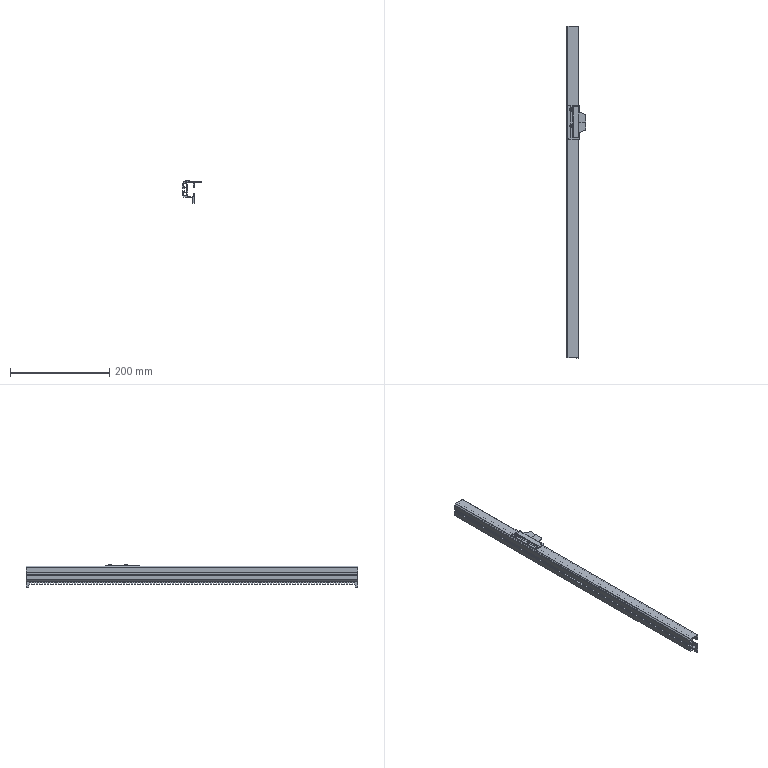Part | STEP file | DEWALT-DWE7492-B22 | 1 solid | 626 faces | box 38.712 x 670 x 45.288 mm | volume 155212 mm3 | plane 572 | cylinder 40 | cone 12 | torus 2 | commonest cylinder face diameters 1 x16 4 x11 2 x8 3.8 x4 4.336 x1